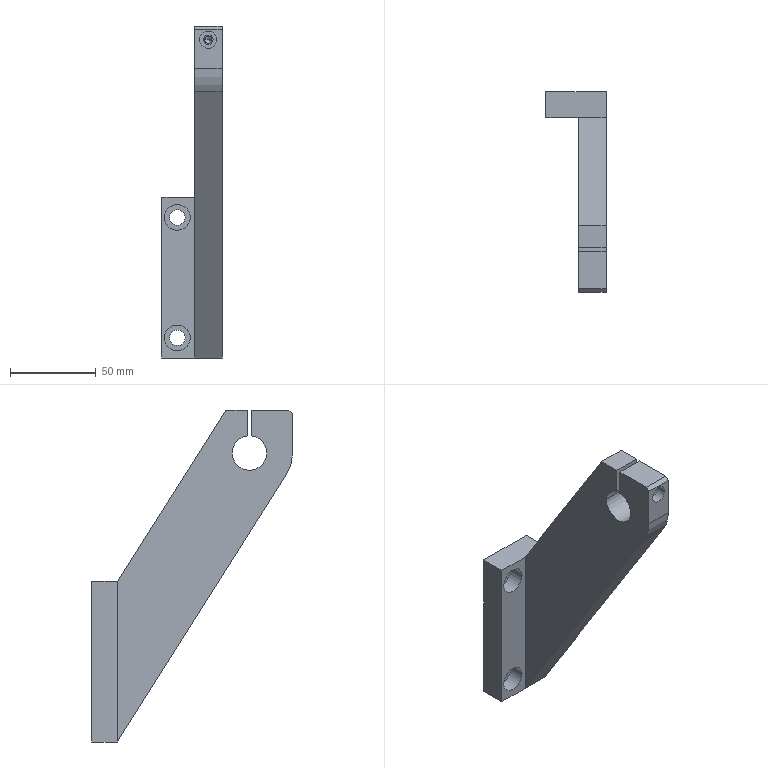Part | NX | features 0004 2 | 1 solid | 38 faces | box 35 x 116.8 x 193.095 mm | volume 171641 mm3 | plane 18 | cylinder 18 | cone 2 | commonest cylinder face diameters 9 x4 15 x4 20 x3 4.2 x2 5.5 x2 10 x2
STEP:
#1=CARTESIAN_POINT('',(-184.3,-184.,-863.625));
#2=VERTEX_POINT('',#1);
#3=CARTESIAN_POINT('',(-168.3,-184.,-863.625));
#4=VERTEX_POINT('',#3);
#5=CARTESIAN_POINT('',(-184.3,-184.,-863.625));
#6=DIRECTION('',(1.,0.,0.));
#7=VECTOR('',#6,1000.);
#8=LINE('',#5,#7);
#9=EDGE_CURVE('',#2,#4,#8,.T.);
#10=ORIENTED_EDGE('',*,*,#9,.T.);
#11=CARTESIAN_POINT('',(-168.3,-281.925,-708.899));
#12=VERTEX_POINT('',#11);
#13=CARTESIAN_POINT('',(-168.3,-281.925,-708.899));
#14=DIRECTION('',(0.,0.5348,-0.845));
#15=VECTOR('',#14,1000.);
#16=LINE('',#13,#15);
#17=EDGE_CURVE('',#12,#4,#16,.T.);
#18=ORIENTED_EDGE('',*,*,#17,.F.);
#19=CARTESIAN_POINT('',(-184.3,-281.925,-708.899));
#20=VERTEX_POINT('',#19);
#21=CARTESIAN_POINT('',(-184.3,-281.925,-708.899));
#22=DIRECTION('',(1.,0.,0.));
#23=VECTOR('',#22,1000.);
#24=LINE('',#21,#23);
#25=EDGE_CURVE('',#20,#12,#24,.T.);
#26=ORIENTED_EDGE('',*,*,#25,.F.);
#27=CARTESIAN_POINT('',(-184.3,-184.,-863.625));
#28=DIRECTION('',(0.,-0.5348,0.845));
#29=VECTOR('',#28,1000.);
#30=LINE('',#27,#29);
#31=EDGE_CURVE('',#2,#20,#30,.T.);
#32=ORIENTED_EDGE('',*,*,#31,.F.);
#33=EDGE_LOOP('',(#10,#18,#26,#32));
#34=FACE_BOUND('',#33,.T.);
#35=CARTESIAN_POINT('',(-168.3,-281.925,-708.899));
#36=DIRECTION('',(0.,0.845,0.5348));
#37=DIRECTION('',(0.,0.5348,-0.845));
#38=AXIS2_PLACEMENT_3D('',#35,#36,#37);
#39=PLANE('',#38);
#40=ADVANCED_FACE('',(#34),#39,.F.);
#41=ORIENTED_EDGE('',*,*,#25,.T.);
#42=CARTESIAN_POINT('',(-168.3,-285.8,-695.529));
#43=VERTEX_POINT('',#42);
#44=CARTESIAN_POINT('',(-168.3,-260.8,-695.529));
#45=DIRECTION('',(1.,0.,0.));
#46=DIRECTION('',(0.,-1.,0.));
#47=AXIS2_PLACEMENT_3D('',#44,#45,#46);
#48=CIRCLE('',#47,25.);
#49=EDGE_CURVE('',#43,#12,#48,.T.);
#50=ORIENTED_EDGE('',*,*,#49,.F.);
#51=CARTESIAN_POINT('',(-184.3,-285.8,-695.529));
#52=VERTEX_POINT('',#51);
#53=CARTESIAN_POINT('',(-168.3,-285.8,-695.529));
#54=DIRECTION('',(-1.,0.,0.));
#55=VECTOR('',#54,1000.);
#56=LINE('',#53,#55);
#57=EDGE_CURVE('',#43,#52,#56,.T.);
#58=ORIENTED_EDGE('',*,*,#57,.T.);
#59=CARTESIAN_POINT('',(-184.3,-260.8,-695.529));
#60=DIRECTION('',(-1.,0.,0.));
#61=DIRECTION('',(0.,-0.845,-0.5348));
#62=AXIS2_PLACEMENT_3D('',#59,#60,#61);
#63=CIRCLE('',#62,25.);
#64=EDGE_CURVE('',#20,#52,#63,.T.);
#65=ORIENTED_EDGE('',*,*,#64,.F.);
#66=EDGE_LOOP('',(#41,#50,#58,#65));
#67=FACE_BOUND('',#66,.T.);
#68=CARTESIAN_POINT('',(-168.3,-260.8,-695.529));
#69=DIRECTION('',(-1.,0.,0.));
#70=DIRECTION('',(0.,1.,0.));
#71=AXIS2_PLACEMENT_3D('',#68,#69,#70);
#72=CYLINDRICAL_SURFACE('',#71,25.);
#73=ADVANCED_FACE('',(#67),#72,.T.);
#74=CARTESIAN_POINT('',(-181.3,-280.1,-678.529));
#75=VERTEX_POINT('',#74);
#76=CARTESIAN_POINT('',(-171.3,-280.1,-678.529));
#77=VERTEX_POINT('',#76);
#78=CARTESIAN_POINT('',(-176.3,-280.1,-678.529));
#79=DIRECTION('',(0.,-1.,0.));
#80=DIRECTION('',(-1.,0.,0.));
#81=AXIS2_PLACEMENT_3D('',#78,#79,#80);
#82=CIRCLE('',#81,5.);
#83=EDGE_CURVE('',#75,#77,#82,.T.);
#84=ORIENTED_EDGE('',*,*,#83,.F.);
#85=CARTESIAN_POINT('',(-181.3,-285.8,-678.529));
#86=VERTEX_POINT('',#85);
#87=CARTESIAN_POINT('',(-181.3,-285.8,-678.529));
#88=DIRECTION('',(0.,1.,0.));
#89=VECTOR('',#88,1000.);
#90=LINE('',#87,#89);
#91=EDGE_CURVE('',#86,#75,#90,.T.);
#92=ORIENTED_EDGE('',*,*,#91,.F.);
#93=CARTESIAN_POINT('',(-171.3,-285.8,-678.529));
#94=VERTEX_POINT('',#93);
#95=CARTESIAN_POINT('',(-176.3,-285.8,-678.529));
#96=DIRECTION('',(0.,1.,0.));
#97=DIRECTION('',(1.,0.,0.));
#98=AXIS2_PLACEMENT_3D('',#95,#96,#97);
#99=CIRCLE('',#98,5.);
#100=EDGE_CURVE('',#94,#86,#99,.T.);
#101=ORIENTED_EDGE('',*,*,#100,.F.);
#102=CARTESIAN_POINT('',(-171.3,-285.8,-678.529));
#103=DIRECTION('',(0.,1.,0.));
#104=VECTOR('',#103,1000.);
#105=LINE('',#102,#104);
#106=EDGE_CURVE('',#77,#94,#105,.F.);
#107=ORIENTED_EDGE('',*,*,#106,.F.);
#108=EDGE_LOOP('',(#84,#92,#101,#107));
#109=FACE_BOUND('',#108,.T.);
#110=CARTESIAN_POINT('',(-176.3,-285.8,-678.529));
#111=DIRECTION('',(0.,-1.,0.));
#112=DIRECTION('',(-1.,0.,0.));
#113=AXIS2_PLACEMENT_3D('',#110,#111,#112);
#114=CYLINDRICAL_SURFACE('',#113,5.);
#115=ADVANCED_FACE('',(#109),#114,.F.);
#116=ORIENTED_EDGE('',*,*,#106,.T.);
#117=CARTESIAN_POINT('',(-176.3,-285.8,-678.529));
#118=DIRECTION('',(0.,1.,0.));
#119=DIRECTION('',(-1.,0.,0.));
#120=AXIS2_PLACEMENT_3D('',#117,#118,#119);
#121=CIRCLE('',#120,5.);
#122=EDGE_CURVE('',#86,#94,#121,.T.);
#123=ORIENTED_EDGE('',*,*,#122,.F.);
#124=ORIENTED_EDGE('',*,*,#91,.T.);
#125=CARTESIAN_POINT('',(-176.3,-280.1,-678.529));
#126=DIRECTION('',(0.,-1.,0.));
#127=DIRECTION('',(1.,0.,0.));
#128=AXIS2_PLACEMENT_3D('',#125,#126,#127);
#129=CIRCLE('',#128,5.);
#130=EDGE_CURVE('',#77,#75,#129,.T.);
#131=ORIENTED_EDGE('',*,*,#130,.F.);
#132=EDGE_LOOP('',(#116,#123,#124,#131));
#133=FACE_BOUND('',#132,.T.);
#134=CARTESIAN_POINT('',(-176.3,-285.8,-678.529));
#135=DIRECTION('',(0.,-1.,0.));
#136=DIRECTION('',(-1.,0.,0.));
#137=AXIS2_PLACEMENT_3D('',#134,#135,#136);
#138=CYLINDRICAL_SURFACE('',#137,5.);
#139=ADVANCED_FACE('',(#133),#138,.F.);
#140=CARTESIAN_POINT('',(-173.55,-280.1,-678.529));
#141=VERTEX_POINT('',#140);
#142=CARTESIAN_POINT('',(-179.05,-280.1,-678.529));
#143=VERTEX_POINT('',#142);
#144=CARTESIAN_POINT('',(-176.3,-280.1,-678.529));
#145=DIRECTION('',(0.,1.,0.));
#146=DIRECTION('',(1.,0.,0.));
#147=AXIS2_PLACEMENT_3D('',#144,#145,#146);
#148=CIRCLE('',#147,2.75);
#149=EDGE_CURVE('',#141,#143,#148,.T.);
#150=ORIENTED_EDGE('',*,*,#149,.T.);
#151=CARTESIAN_POINT('',(-176.3,-280.1,-678.529));
#152=DIRECTION('',(0.,1.,0.));
#153=DIRECTION('',(-1.,0.,0.));
#154=AXIS2_PLACEMENT_3D('',#151,#152,#153);
#155=CIRCLE('',#154,2.75);
#156=EDGE_CURVE('',#143,#141,#155,.T.);
#157=ORIENTED_EDGE('',*,*,#156,.T.);
#158=EDGE_LOOP('',(#150,#157));
#159=FACE_BOUND('',#158,.T.);
#160=ORIENTED_EDGE('',*,*,#83,.T.);
#161=ORIENTED_EDGE('',*,*,#130,.T.);
#162=EDGE_LOOP('',(#160,#161));
#163=FACE_BOUND('',#162,.T.);
#164=CARTESIAN_POINT('',(-176.3,-280.1,-675.779));
#165=DIRECTION('',(0.,1.,0.));
#166=DIRECTION('',(1.,0.,0.));
#167=AXIS2_PLACEMENT_3D('',#164,#165,#166);
#168=PLANE('',#167);
#169=ADVANCED_FACE('',(#159,#163),#168,.F.);
#170=CARTESIAN_POINT('',(-173.55,-262.05,-678.529));
#171=VERTEX_POINT('',#170);
#172=CARTESIAN_POINT('',(-173.55,-280.1,-678.529));
#173=DIRECTION('',(0.,1.,0.));
#174=VECTOR('',#173,1000.);
#175=LINE('',#172,#174);
#176=EDGE_CURVE('',#171,#141,#175,.F.);
#177=ORIENTED_EDGE('',*,*,#176,.T.);
#178=ORIENTED_EDGE('',*,*,#156,.F.);
#179=CARTESIAN_POINT('',(-179.05,-262.05,-678.529));
#180=VERTEX_POINT('',#179);
#181=CARTESIAN_POINT('',(-179.05,-280.1,-678.529));
#182=DIRECTION('',(0.,1.,0.));
#183=VECTOR('',#182,1000.);
#184=LINE('',#181,#183);
#185=EDGE_CURVE('',#143,#180,#184,.T.);
#186=ORIENTED_EDGE('',*,*,#185,.T.);
#187=CARTESIAN_POINT('',(-176.3,-262.05,-678.529));
#188=DIRECTION('',(0.,-1.,0.));
#189=DIRECTION('',(1.,0.,0.));
#190=AXIS2_PLACEMENT_3D('',#187,#188,#189);
#191=CIRCLE('',#190,2.75);
#192=EDGE_CURVE('',#171,#180,#191,.T.);
#193=ORIENTED_EDGE('',*,*,#192,.F.);
#194=EDGE_LOOP('',(#177,#178,#186,#193));
#195=FACE_BOUND('',#194,.T.);
#196=CARTESIAN_POINT('',(-176.3,-285.8,-678.529));
#197=DIRECTION('',(0.,-1.,0.));
#198=DIRECTION('',(-1.,0.,0.));
#199=AXIS2_PLACEMENT_3D('',#196,#197,#198);
#200=CYLINDRICAL_SURFACE('',#199,2.75);
#201=ADVANCED_FACE('',(#195),#200,.F.);
#202=CARTESIAN_POINT('',(-176.3,-262.05,-678.529));
#203=DIRECTION('',(0.,-1.,0.));
#204=DIRECTION('',(-1.,0.,0.));
#205=AXIS2_PLACEMENT_3D('',#202,#203,#204);
#206=CIRCLE('',#205,2.75);
#207=EDGE_CURVE('',#180,#171,#206,.T.);
#208=ORIENTED_EDGE('',*,*,#207,.F.);
#209=ORIENTED_EDGE('',*,*,#185,.F.);
#210=ORIENTED_EDGE('',*,*,#149,.F.);
#211=ORIENTED_EDGE('',*,*,#176,.F.);
#212=EDGE_LOOP('',(#208,#209,#210,#211));
#213=FACE_BOUND('',#212,.T.);
#214=CARTESIAN_POINT('',(-176.3,-285.8,-678.529));
#215=DIRECTION('',(0.,-1.,0.));
#216=DIRECTION('',(-1.,0.,0.));
#217=AXIS2_PLACEMENT_3D('',#214,#215,#216);
#218=CYLINDRICAL_SURFACE('',#217,2.75);
#219=ADVANCED_FACE('',(#213),#218,.F.);
#220=CARTESIAN_POINT('',(-178.4,-247.15,-678.529));
#221=VERTEX_POINT('',#220);
#222=CARTESIAN_POINT('',(-174.2,-247.15,-678.529));
#223=VERTEX_POINT('',#222);
#224=CARTESIAN_POINT('',(-176.3,-247.15,-678.529));
#225=DIRECTION('',(0.,-1.,0.));
#226=DIRECTION('',(-1.,0.,0.));
#227=AXIS2_PLACEMENT_3D('',#224,#225,#226);
#228=CIRCLE('',#227,2.1);
#229=EDGE_CURVE('',#221,#223,#228,.T.);
#230=ORIENTED_EDGE('',*,*,#229,.F.);
#231=CARTESIAN_POINT('',(-178.4,-259.55,-678.529));
#232=VERTEX_POINT('',#231);
#233=CARTESIAN_POINT('',(-178.4,-259.55,-678.529));
#234=DIRECTION('',(0.,1.,0.));
#235=VECTOR('',#234,1000.);
#236=LINE('',#233,#235);
#237=EDGE_CURVE('',#232,#221,#236,.T.);
#238=ORIENTED_EDGE('',*,*,#237,.F.);
#239=CARTESIAN_POINT('',(-174.2,-259.55,-678.529));
#240=VERTEX_POINT('',#239);
#241=CARTESIAN_POINT('',(-176.3,-259.55,-678.529));
#242=DIRECTION('',(0.,1.,0.));
#243=DIRECTION('',(1.,0.,0.));
#244=AXIS2_PLACEMENT_3D('',#241,#242,#243);
#245=CIRCLE('',#244,2.1);
#246=EDGE_CURVE('',#240,#232,#245,.T.);
#247=ORIENTED_EDGE('',*,*,#246,.F.);
#248=CARTESIAN_POINT('',(-174.2,-259.55,-678.529));
#249=DIRECTION('',(0.,1.,0.));
#250=VECTOR('',#249,1000.);
#251=LINE('',#248,#250);
#252=EDGE_CURVE('',#223,#240,#251,.F.);
#253=ORIENTED_EDGE('',*,*,#252,.F.);
#254=EDGE_LOOP('',(#230,#238,#247,#253));
#255=FACE_BOUND('',#254,.T.);
#256=CARTESIAN_POINT('',(-176.3,-259.55,-678.529));
#257=DIRECTION('',(0.,-1.,0.));
#258=DIRECTION('',(-1.,0.,0.));
#259=AXIS2_PLACEMENT_3D('',#256,#257,#258);
#260=CYLINDRICAL_SURFACE('',#259,2.1);
#261=ADVANCED_FACE('',(#255),#260,.F.);
#262=CARTESIAN_POINT('',(-176.3,-245.888,-678.529));
#263=VERTEX_POINT('',#262);
#264=CARTESIAN_POINT('',(-178.4,-247.15,-678.529));
#265=DIRECTION('',(0.8572,0.515,0.));
#266=VECTOR('',#265,1000.);
#267=LINE('',#264,#266);
#268=EDGE_CURVE('',#263,#221,#267,.F.);
#269=ORIENTED_EDGE('',*,*,#268,.T.);
#270=ORIENTED_EDGE('',*,*,#229,.T.);
#271=CARTESIAN_POINT('',(-174.2,-247.15,-678.529));
#272=DIRECTION('',(-0.8572,0.515,0.));
#273=VECTOR('',#272,1000.);
#274=LINE('',#271,#273);
#275=EDGE_CURVE('',#223,#263,#274,.T.);
#276=ORIENTED_EDGE('',*,*,#275,.T.);
#277=EDGE_LOOP('',(#269,#270,#276));
#278=FACE_BOUND('',#277,.T.);
#279=CARTESIAN_POINT('',(-176.3,-245.888,-678.529));
#280=DIRECTION('',(0.,-1.,0.));
#281=DIRECTION('',(-1.,0.,0.));
#282=AXIS2_PLACEMENT_3D('',#279,#280,#281);
#283=CONICAL_SURFACE('',#282,0.,1.03);
#284=ADVANCED_FACE('',(#278),#283,.F.);
#285=ORIENTED_EDGE('',*,*,#275,.F.);
#286=CARTESIAN_POINT('',(-176.3,-247.15,-678.529));
#287=DIRECTION('',(0.,-1.,0.));
#288=DIRECTION('',(1.,0.,0.));
#289=AXIS2_PLACEMENT_3D('',#286,#287,#288);
#290=CIRCLE('',#289,2.1);
#291=EDGE_CURVE('',#223,#221,#290,.T.);
#292=ORIENTED_EDGE('',*,*,#291,.T.);
#293=ORIENTED_EDGE('',*,*,#268,.F.);
#294=EDGE_LOOP('',(#285,#292,#293));
#295=FACE_BOUND('',#294,.T.);
#296=CARTESIAN_POINT('',(-176.3,-245.888,-678.529));
#297=DIRECTION('',(0.,-1.,0.));
#298=DIRECTION('',(-1.,0.,0.));
#299=AXIS2_PLACEMENT_3D('',#296,#297,#298);
#300=CONICAL_SURFACE('',#299,0.,1.03);
#301=ADVANCED_FACE('',(#295),#300,.F.);
#302=ORIENTED_EDGE('',*,*,#252,.T.);
#303=CARTESIAN_POINT('',(-176.3,-259.55,-678.529));
#304=DIRECTION('',(0.,1.,0.));
#305=DIRECTION('',(-1.,0.,0.));
#306=AXIS2_PLACEMENT_3D('',#303,#304,#305);
#307=CIRCLE('',#306,2.1);
#308=EDGE_CURVE('',#232,#240,#307,.T.);
#309=ORIENTED_EDGE('',*,*,#308,.F.);
#310=ORIENTED_EDGE('',*,*,#237,.T.);
#311=ORIENTED_EDGE('',*,*,#291,.F.);
#312=EDGE_LOOP('',(#302,#309,#310,#311));
#313=FACE_BOUND('',#312,.T.);
#314=CARTESIAN_POINT('',(-176.3,-259.55,-678.529));
#315=DIRECTION('',(0.,-1.,0.));
#316=DIRECTION('',(-1.,0.,0.));
#317=AXIS2_PLACEMENT_3D('',#314,#315,#316);
#318=CYLINDRICAL_SURFACE('',#317,2.1);
#319=ADVANCED_FACE('',(#313),#318,.F.);
#320=CARTESIAN_POINT('',(-201.8,-175.,-781.877));
#321=VERTEX_POINT('',#320);
#322=CARTESIAN_POINT('',(-186.8,-175.,-781.877));
#323=VERTEX_POINT('',#322);
#324=CARTESIAN_POINT('',(-194.3,-175.,-781.877));
#325=DIRECTION('',(0.,-1.,0.));
#326=DIRECTION('',(-1.,0.,0.));
#327=AXIS2_PLACEMENT_3D('',#324,#325,#326);
#328=CIRCLE('',#327,7.5);
#329=EDGE_CURVE('',#321,#323,#328,.T.);
#330=ORIENTED_EDGE('',*,*,#329,.F.);
#331=CARTESIAN_POINT('',(-201.8,-184.,-781.877));
#332=VERTEX_POINT('',#331);
#333=CARTESIAN_POINT('',(-201.8,-184.,-781.877));
#334=DIRECTION('',(0.,1.,0.));
#335=VECTOR('',#334,1000.);
#336=LINE('',#333,#335);
#337=EDGE_CURVE('',#332,#321,#336,.T.);
#338=ORIENTED_EDGE('',*,*,#337,.F.);
#339=CARTESIAN_POINT('',(-186.8,-184.,-781.877));
#340=VERTEX_POINT('',#339);
#341=CARTESIAN_POINT('',(-194.3,-184.,-781.877));
#342=DIRECTION('',(0.,1.,0.));
#343=DIRECTION('',(1.,0.,0.));
#344=AXIS2_PLACEMENT_3D('',#341,#342,#343);
#345=CIRCLE('',#344,7.5);
#346=EDGE_CURVE('',#340,#332,#345,.T.);
#347=ORIENTED_EDGE('',*,*,#346,.F.);
#348=CARTESIAN_POINT('',(-186.8,-184.,-781.877));
#349=DIRECTION('',(0.,1.,0.));
#350=VECTOR('',#349,1000.);
#351=LINE('',#348,#350);
#352=EDGE_CURVE('',#323,#340,#351,.F.);
#353=ORIENTED_EDGE('',*,*,#352,.F.);
#354=EDGE_LOOP('',(#330,#338,#347,#353));
#355=FACE_BOUND('',#354,.T.);
#356=CARTESIAN_POINT('',(-194.3,-184.,-781.877));
#357=DIRECTION('',(0.,-1.,0.));
#358=DIRECTION('',(-1.,0.,0.));
#359=AXIS2_PLACEMENT_3D('',#356,#357,#358);
#360=CYLINDRICAL_SURFACE('',#359,7.5);
#361=ADVANCED_FACE('',(#355),#360,.F.);
#362=ORIENTED_EDGE('',*,*,#352,.T.);
#363=CARTESIAN_POINT('',(-194.3,-184.,-781.877));
#364=DIRECTION('',(0.,1.,0.));
#365=DIRECTION('',(-1.,0.,0.));
#366=AXIS2_PLACEMENT_3D('',#363,#364,#365);
#367=CIRCLE('',#366,7.5);
#368=EDGE_CURVE('',#332,#340,#367,.T.);
#369=ORIENTED_EDGE('',*,*,#368,.F.);
#370=ORIENTED_EDGE('',*,*,#337,.T.);
#371=CARTESIAN_POINT('',(-194.3,-175.,-781.877));
#372=DIRECTION('',(0.,-1.,0.));
#373=DIRECTION('',(1.,0.,0.));
#374=AXIS2_PLACEMENT_3D('',#371,#372,#373);
#375=CIRCLE('',#374,7.5);
#376=EDGE_CURVE('',#323,#321,#375,.T.);
#377=ORIENTED_EDGE('',*,*,#376,.F.);
#378=EDGE_LOOP('',(#362,#369,#370,#377));
#379=FACE_BOUND('',#378,.T.);
#380=CARTESIAN_POINT('',(-194.3,-184.,-781.877));
#381=DIRECTION('',(0.,-1.,0.));
#382=DIRECTION('',(-1.,0.,0.));
#383=AXIS2_PLACEMENT_3D('',#380,#381,#382);
#384=CYLINDRICAL_SURFACE('',#383,7.5);
#385=ADVANCED_FACE('',(#379),#384,.F.);
#386=CARTESIAN_POINT('',(-189.8,-175.,-781.877));
#387=VERTEX_POINT('',#386);
#388=CARTESIAN_POINT('',(-198.8,-175.,-781.877));
#389=VERTEX_POINT('',#388);
#390=CARTESIAN_POINT('',(-194.3,-175.,-781.877));
#391=DIRECTION('',(0.,1.,0.));
#392=DIRECTION('',(1.,0.,0.));
#393=AXIS2_PLACEMENT_3D('',#390,#391,#392);
#394=CIRCLE('',#393,4.5);
#395=EDGE_CURVE('',#387,#389,#394,.T.);
#396=ORIENTED_EDGE('',*,*,#395,.T.);
#397=CARTESIAN_POINT('',(-194.3,-175.,-781.877));
#398=DIRECTION('',(0.,1.,0.));
#399=DIRECTION('',(-1.,0.,0.));
#400=AXIS2_PLACEMENT_3D('',#397,#398,#399);
#401=CIRCLE('',#400,4.5);
#402=EDGE_CURVE('',#389,#387,#401,.T.);
#403=ORIENTED_EDGE('',*,*,#402,.T.);
#404=EDGE_LOOP('',(#396,#403));
#405=FACE_BOUND('',#404,.T.);
#406=ORIENTED_EDGE('',*,*,#329,.T.);
#407=ORIENTED_EDGE('',*,*,#376,.T.);
#408=EDGE_LOOP('',(#406,#407));
#409=FACE_BOUND('',#408,.T.);
#410=CARTESIAN_POINT('',(-194.3,-175.,-777.377));
#411=DIRECTION('',(0.,1.,0.));
#412=DIRECTION('',(1.,0.,0.));
#413=AXIS2_PLACEMENT_3D('',#410,#411,#412);
#414=PLANE('',#413);
#415=ADVANCED_FACE('',(#405,#409),#414,.F.);
#416=CARTESIAN_POINT('',(-198.8,-169.,-781.877));
#417=VERTEX_POINT('',#416);
#418=CARTESIAN_POINT('',(-189.8,-169.,-781.877));
#419=VERTEX_POINT('',#418);
#420=CARTESIAN_POINT('',(-194.3,-169.,-781.877));
#421=DIRECTION('',(0.,-1.,0.));
#422=DIRECTION('',(-1.,0.,0.));
#423=AXIS2_PLACEMENT_3D('',#420,#421,#422);
#424=CIRCLE('',#423,4.5);
#425=EDGE_CURVE('',#417,#419,#424,.T.);
#426=ORIENTED_EDGE('',*,*,#425,.F.);
#427=CARTESIAN_POINT('',(-198.8,-175.,-781.877));
#428=DIRECTION('',(0.,1.,0.));
#429=VECTOR('',#428,1000.);
#430=LINE('',#427,#429);
#431=EDGE_CURVE('',#417,#389,#430,.F.);
#432=ORIENTED_EDGE('',*,*,#431,.T.);
#433=ORIENTED_EDGE('',*,*,#395,.F.);
#434=CARTESIAN_POINT('',(-189.8,-175.,-781.877));
#435=DIRECTION('',(0.,1.,0.));
#436=VECTOR('',#435,1000.);
#437=LINE('',#434,#436);
#438=EDGE_CURVE('',#387,#419,#437,.T.);
#439=ORIENTED_EDGE('',*,*,#438,.T.);
#440=EDGE_LOOP('',(#426,#432,#433,#439));
#441=FACE_BOUND('',#440,.T.);
#442=CARTESIAN_POINT('',(-194.3,-184.,-781.877));
#443=DIRECTION('',(0.,-1.,0.));
#444=DIRECTION('',(-1.,0.,0.));
#445=AXIS2_PLACEMENT_3D('',#442,#443,#444);
#446=CYLINDRICAL_SURFACE('',#445,4.5);
#447=ADVANCED_FACE('',(#441),#446,.F.);
#448=ORIENTED_EDGE('',*,*,#438,.F.);
#449=ORIENTED_EDGE('',*,*,#402,.F.);
#450=ORIENTED_EDGE('',*,*,#431,.F.);
#451=CARTESIAN_POINT('',(-194.3,-169.,-781.877));
#452=DIRECTION('',(0.,-1.,0.));
#453=DIRECTION('',(1.,0.,0.));
#454=AXIS2_PLACEMENT_3D('',#451,#452,#453);
#455=CIRCLE('',#454,4.5);
#456=EDGE_CURVE('',#419,#417,#455,.T.);
#457=ORIENTED_EDGE('',*,*,#456,.F.);
#458=EDGE_LOOP('',(#448,#449,#450,#457));
#459=FACE_BOUND('',#458,.T.);
#460=CARTESIAN_POINT('',(-194.3,-184.,-781.877));
#461=DIRECTION('',(0.,-1.,0.));
#462=DIRECTION('',(-1.,0.,0.));
#463=AXIS2_PLACEMENT_3D('',#460,#461,#462);
#464=CYLINDRICAL_SURFACE('',#463,4.5);
#465=ADVANCED_FACE('',(#459),#464,.F.);
#466=CARTESIAN_POINT('',(-201.8,-175.,-851.877));
#467=VERTEX_POINT('',#466);
#468=CARTESIAN_POINT('',(-186.8,-175.,-851.877));
#469=VERTEX_POINT('',#468);
#470=CARTESIAN_POINT('',(-194.3,-175.,-851.877));
#471=DIRECTION('',(0.,-1.,0.));
#472=DIRECTION('',(-1.,0.,0.));
#473=AXIS2_PLACEMENT_3D('',#470,#471,#472);
#474=CIRCLE('',#473,7.5);
#475=EDGE_CURVE('',#467,#469,#474,.T.);
#476=ORIENTED_EDGE('',*,*,#475,.F.);
#477=CARTESIAN_POINT('',(-201.8,-184.,-851.877));
#478=VERTEX_POINT('',#477);
#479=CARTESIAN_POINT('',(-201.8,-184.,-851.877));
#480=DIRECTION('',(0.,1.,0.));
#481=VECTOR('',#480,1000.);
#482=LINE('',#479,#481);
#483=EDGE_CURVE('',#467,#478,#482,.F.);
#484=ORIENTED_EDGE('',*,*,#483,.T.);
#485=CARTESIAN_POINT('',(-186.8,-184.,-851.877));
#486=VERTEX_POINT('',#485);
#487=CARTESIAN_POINT('',(-194.3,-184.,-851.877));
#488=DIRECTION('',(0.,1.,0.));
#489=DIRECTION('',(1.,0.,0.));
#490=AXIS2_PLACEMENT_3D('',#487,#488,#489);
#491=CIRCLE('',#490,7.5);
#492=EDGE_CURVE('',#486,#478,#491,.T.);
#493=ORIENTED_EDGE('',*,*,#492,.F.);
#494=CARTESIAN_POINT('',(-186.8,-184.,-851.877));
#495=DIRECTION('',(0.,1.,0.));
#496=VECTOR('',#495,1000.);
#497=LINE('',#494,#496);
#498=EDGE_CURVE('',#486,#469,#497,.T.);
#499=ORIENTED_EDGE('',*,*,#498,.T.);
#500=EDGE_LOOP('',(#476,#484,#493,#499));
#501=FACE_BOUND('',#500,.T.);
#502=CARTESIAN_POINT('',(-194.3,-184.,-851.877));
#503=DIRECTION('',(0.,-1.,0.));
#504=DIRECTION('',(-1.,0.,0.));
#505=AXIS2_PLACEMENT_3D('',#502,#503,#504);
#506=CYLINDRICAL_SURFACE('',#505,7.5);
#507=ADVANCED_FACE('',(#501),#506,.F.);
#508=ORIENTED_EDGE('',*,*,#498,.F.);
#509=CARTESIAN_POINT('',(-194.3,-184.,-851.877));
#510=DIRECTION('',(0.,1.,0.));
#511=DIRECTION('',(-1.,0.,0.));
#512=AXIS2_PLACEMENT_3D('',#509,#510,#511);
#513=CIRCLE('',#512,7.5);
#514=EDGE_CURVE('',#478,#486,#513,.T.);
#515=ORIENTED_EDGE('',*,*,#514,.F.);
#516=ORIENTED_EDGE('',*,*,#483,.F.);
#517=CARTESIAN_POINT('',(-194.3,-175.,-851.877));
#518=DIRECTION('',(0.,-1.,0.));
#519=DIRECTION('',(1.,0.,0.));
#520=AXIS2_PLACEMENT_3D('',#517,#518,#519);
#521=CIRCLE('',#520,7.5);
#522=EDGE_CURVE('',#469,#467,#521,.T.);
#523=ORIENTED_EDGE('',*,*,#522,.F.);
#524=EDGE_LOOP('',(#508,#515,#516,#523));
#525=FACE_BOUND('',#524,.T.);
#526=CARTESIAN_POINT('',(-194.3,-184.,-851.877));
#527=DIRECTION('',(0.,-1.,0.));
#528=DIRECTION('',(-1.,0.,0.));
#529=AXIS2_PLACEMENT_3D('',#526,#527,#528);
#530=CYLINDRICAL_SURFACE('',#529,7.5);
#531=ADVANCED_FACE('',(#525),#530,.F.);
#532=CARTESIAN_POINT('',(-189.8,-175.,-851.877));
#533=VERTEX_POINT('',#532);
#534=CARTESIAN_POINT('',(-198.8,-175.,-851.877));
#535=VERTEX_POINT('',#534);
#536=CARTESIAN_POINT('',(-194.3,-175.,-851.877));
#537=DIRECTION('',(0.,1.,0.));
#538=DIRECTION('',(1.,0.,0.));
#539=AXIS2_PLACEMENT_3D('',#536,#537,#538);
#540=CIRCLE('',#539,4.5);
#541=EDGE_CURVE('',#533,#535,#540,.T.);
#542=ORIENTED_EDGE('',*,*,#541,.T.);
#543=CARTESIAN_POINT('',(-194.3,-175.,-851.877));
#544=DIRECTION('',(0.,1.,0.));
#545=DIRECTION('',(-1.,0.,0.));
#546=AXIS2_PLACEMENT_3D('',#543,#544,#545);
#547=CIRCLE('',#546,4.5);
#548=EDGE_CURVE('',#535,#533,#547,.T.);
#549=ORIENTED_EDGE('',*,*,#548,.T.);
#550=EDGE_LOOP('',(#542,#549));
#551=FACE_BOUND('',#550,.T.);
#552=ORIENTED_EDGE('',*,*,#475,.T.);
#553=ORIENTED_EDGE('',*,*,#522,.T.);
#554=EDGE_LOOP('',(#552,#553));
#555=FACE_BOUND('',#554,.T.);
#556=CARTESIAN_POINT('',(-194.3,-175.,-847.377));
#557=DIRECTION('',(0.,1.,0.));
#558=DIRECTION('',(1.,0.,0.));
#559=AXIS2_PLACEMENT_3D('',#556,#557,#558);
#560=PLANE('',#559);
#561=ADVANCED_FACE('',(#551,#555),#560,.F.);
#562=CARTESIAN_POINT('',(-198.8,-169.,-851.877));
#563=VERTEX_POINT('',#562);
#564=CARTESIAN_POINT('',(-189.8,-169.,-851.877));
#565=VERTEX_POINT('',#564);
#566=CARTESIAN_POINT('',(-194.3,-169.,-851.877));
#567=DIRECTION('',(0.,-1.,0.));
#568=DIRECTION('',(-1.,0.,0.));
#569=AXIS2_PLACEMENT_3D('',#566,#567,#568);
#570=CIRCLE('',#569,4.5);
#571=EDGE_CURVE('',#563,#565,#570,.T.);
#572=ORIENTED_EDGE('',*,*,#571,.F.);
#573=CARTESIAN_POINT('',(-198.8,-175.,-851.877));
#574=DIRECTION('',(0.,1.,0.));
#575=VECTOR('',#574,1000.);
#576=LINE('',#573,#575);
#577=EDGE_CURVE('',#535,#563,#576,.T.);
#578=ORIENTED_EDGE('',*,*,#577,.F.);
#579=ORIENTED_EDGE('',*,*,#541,.F.);
#580=CARTESIAN_POINT('',(-189.8,-175.,-851.877));
#581=DIRECTION('',(0.,1.,0.));
#582=VECTOR('',#581,1000.);
#583=LINE('',#580,#582);
#584=EDGE_CURVE('',#565,#533,#583,.F.);
#585=ORIENTED_EDGE('',*,*,#584,.F.);
#586=EDGE_LOOP('',(#572,#578,#579,#585));
#587=FACE_BOUND('',#586,.T.);
#588=CARTESIAN_POINT('',(-194.3,-184.,-851.877));
#589=DIRECTION('',(0.,-1.,0.));
#590=DIRECTION('',(-1.,0.,0.));
#591=AXIS2_PLACEMENT_3D('',#588,#589,#590);
#592=CYLINDRICAL_SURFACE('',#591,4.5);
#593=ADVANCED_FACE('',(#587),#592,.F.);
#594=ORIENTED_EDGE('',*,*,#584,.T.);
#595=ORIENTED_EDGE('',*,*,#548,.F.);
#596=ORIENTED_EDGE('',*,*,#577,.T.);
#597=CARTESIAN_POINT('',(-194.3,-169.,-851.877));
#598=DIRECTION('',(0.,-1.,0.));
#599=DIRECTION('',(1.,0.,0.));
#600=AXIS2_PLACEMENT_3D('',#597,#598,#599);
#601=CIRCLE('',#600,4.5);
#602=EDGE_CURVE('',#565,#563,#601,.T.);
#603=ORIENTED_EDGE('',*,*,#602,.F.);
#604=EDGE_LOOP('',(#594,#595,#596,#603));
#605=FACE_BOUND('',#604,.T.);
#606=CARTESIAN_POINT('',(-194.3,-184.,-851.877));
#607=DIRECTION('',(0.,-1.,0.));
#608=DIRECTION('',(-1.,0.,0.));
#609=AXIS2_PLACEMENT_3D('',#606,#607,#608);
#610=CYLINDRICAL_SURFACE('',#609,4.5);
#611=ADVANCED_FACE('',(#605),#610,.F.);
#612=ORIENTED_EDGE('',*,*,#425,.T.);
#613=ORIENTED_EDGE('',*,*,#456,.T.);
#614=EDGE_LOOP('',(#612,#613));
#615=FACE_BOUND('',#614,.T.);
#616=ORIENTED_EDGE('',*,*,#571,.T.);
#617=ORIENTED_EDGE('',*,*,#602,.T.);
#618=EDGE_LOOP('',(#616,#617));
#619=FACE_BOUND('',#618,.T.);
#620=CARTESIAN_POINT('',(-168.3,-169.,-863.625));
#621=VERTEX_POINT('',#620);
#622=CARTESIAN_POINT('',(-203.3,-169.,-863.625));
#623=VERTEX_POINT('',#622);
#624=CARTESIAN_POINT('',(-168.3,-169.,-863.625));
#625=DIRECTION('',(-1.,0.,0.));
#626=VECTOR('',#625,1000.);
#627=LINE('',#624,#626);
#628=EDGE_CURVE('',#621,#623,#627,.T.);
#629=ORIENTED_EDGE('',*,*,#628,.T.);
#630=CARTESIAN_POINT('',(-203.3,-169.,-770.129));
#631=VERTEX_POINT('',#630);
#632=CARTESIAN_POINT('',(-203.3,-169.,-863.625));
#633=DIRECTION('',(0.,0.,1.));
#634=VECTOR('',#633,1000.);
#635=LINE('',#632,#634);
#636=EDGE_CURVE('',#623,#631,#635,.T.);
#637=ORIENTED_EDGE('',*,*,#636,.T.);
#638=CARTESIAN_POINT('',(-168.3,-169.,-770.129));
#639=VERTEX_POINT('',#638);
#640=CARTESIAN_POINT('',(-168.3,-169.,-770.129));
#641=DIRECTION('',(-1.,0.,0.));
#642=VECTOR('',#641,1000.);
#643=LINE('',#640,#642);
#644=EDGE_CURVE('',#639,#631,#643,.T.);
#645=ORIENTED_EDGE('',*,*,#644,.F.);
#646=CARTESIAN_POINT('',(-168.3,-169.,-863.625));
#647=DIRECTION('',(0.,0.,1.));
#648=VECTOR('',#647,1000.);
#649=LINE('',#646,#648);
#650=EDGE_CURVE('',#621,#639,#649,.T.);
#651=ORIENTED_EDGE('',*,*,#650,.F.);
#652=EDGE_LOOP('',(#629,#637,#645,#651));
#653=FACE_BOUND('',#652,.T.);
#654=CARTESIAN_POINT('',(-203.3,-169.,-770.129));
#655=DIRECTION('',(0.,1.,0.));
#656=DIRECTION('',(1.,0.,0.));
#657=AXIS2_PLACEMENT_3D('',#654,#655,#656);
#658=PLANE('',#657);
#659=ADVANCED_FACE('',(#615,#619,#653),#658,.T.);
#660=CARTESIAN_POINT('',(-203.3,-184.,-863.625));
#661=VERTEX_POINT('',#660);
#662=CARTESIAN_POINT('',(-203.3,-184.,-863.625));
#663=DIRECTION('',(0.,1.,0.));
#664=VECTOR('',#663,1000.);
#665=LINE('',#662,#664);
#666=EDGE_CURVE('',#661,#623,#665,.T.);
#667=ORIENTED_EDGE('',*,*,#666,.F.);
#668=CARTESIAN_POINT('',(-203.3,-184.,-770.129));
#669=VERTEX_POINT('',#668);
#670=CARTESIAN_POINT('',(-203.3,-184.,-770.129));
#671=DIRECTION('',(0.,0.,-1.));
#672=VECTOR('',#671,1000.);
#673=LINE('',#670,#672);
#674=EDGE_CURVE('',#669,#661,#673,.T.);
#675=ORIENTED_EDGE('',*,*,#674,.F.);
#676=CARTESIAN_POINT('',(-203.3,-169.,-770.129));
#677=DIRECTION('',(0.,-1.,0.));
#678=VECTOR('',#677,1000.);
#679=LINE('',#676,#678);
#680=EDGE_CURVE('',#631,#669,#679,.T.);
#681=ORIENTED_EDGE('',*,*,#680,.F.);
#682=ORIENTED_EDGE('',*,*,#636,.F.);
#683=EDGE_LOOP('',(#667,#675,#681,#682));
#684=FACE_BOUND('',#683,.T.);
#685=CARTESIAN_POINT('',(-203.3,-169.,-770.129));
#686=DIRECTION('',(1.,0.,0.));
#687=DIRECTION('',(0.,-1.,0.));
#688=AXIS2_PLACEMENT_3D('',#685,#686,#687);
#689=PLANE('',#688);
#690=ADVANCED_FACE('',(#684),#689,.F.);
#691=ORIENTED_EDGE('',*,*,#492,.T.);
#692=ORIENTED_EDGE('',*,*,#514,.T.);
#693=EDGE_LOOP('',(#691,#692));
#694=FACE_BOUND('',#693,.T.);
#695=ORIENTED_EDGE('',*,*,#346,.T.);
#696=ORIENTED_EDGE('',*,*,#368,.T.);
#697=EDGE_LOOP('',(#695,#696));
#698=FACE_BOUND('',#697,.T.);
#699=ORIENTED_EDGE('',*,*,#674,.T.);
#700=CARTESIAN_POINT('',(-184.3,-184.,-863.625));
#701=DIRECTION('',(-1.,0.,0.));
#702=VECTOR('',#701,1000.);
#703=LINE('',#700,#702);
#704=EDGE_CURVE('',#2,#661,#703,.T.);
#705=ORIENTED_EDGE('',*,*,#704,.F.);
#706=CARTESIAN_POINT('',(-184.3,-184.,-770.129));
#707=VERTEX_POINT('',#706);
#708=CARTESIAN_POINT('',(-184.3,-184.,-863.625));
#709=DIRECTION('',(0.,0.,1.));
#710=VECTOR('',#709,1000.);
#711=LINE('',#708,#710);
#712=EDGE_CURVE('',#2,#707,#711,.T.);
#713=ORIENTED_EDGE('',*,*,#712,.T.);
#714=CARTESIAN_POINT('',(-184.3,-184.,-770.129));
#715=DIRECTION('',(-1.,0.,0.));
#716=VECTOR('',#715,1000.);
#717=LINE('',#714,#716);
#718=EDGE_CURVE('',#707,#669,#717,.T.);
#719=ORIENTED_EDGE('',*,*,#718,.T.);
#720=EDGE_LOOP('',(#699,#705,#713,#719));
#721=FACE_BOUND('',#720,.T.);
#722=CARTESIAN_POINT('',(-203.3,-184.,-770.129));
#723=DIRECTION('',(0.,-1.,0.));
#724=DIRECTION('',(-1.,0.,0.));
#725=AXIS2_PLACEMENT_3D('',#722,#723,#724);
#726=PLANE('',#725);
#727=ADVANCED_FACE('',(#694,#698,#721),#726,.T.);
#728=ORIENTED_EDGE('',*,*,#644,.T.);
#729=ORIENTED_EDGE('',*,*,#680,.T.);
#730=ORIENTED_EDGE('',*,*,#718,.F.);
#731=CARTESIAN_POINT('',(-168.3,-184.,-770.129));
#732=VERTEX_POINT('',#731);
#733=CARTESIAN_POINT('',(-184.3,-184.,-770.129));
#734=DIRECTION('',(1.,0.,0.));
#735=VECTOR('',#734,1000.);
#736=LINE('',#733,#735);
#737=EDGE_CURVE('',#707,#732,#736,.T.);
#738=ORIENTED_EDGE('',*,*,#737,.T.);
#739=CARTESIAN_POINT('',(-168.3,-169.,-770.129));
#740=DIRECTION('',(0.,-1.,0.));
#741=VECTOR('',#740,1000.);
#742=LINE('',#739,#741);
#743=EDGE_CURVE('',#639,#732,#742,.T.);
#744=ORIENTED_EDGE('',*,*,#743,.F.);
#745=EDGE_LOOP('',(#728,#729,#730,#738,#744));
#746=FACE_BOUND('',#745,.T.);
#747=CARTESIAN_POINT('',(-203.3,-169.,-770.129));
#748=DIRECTION('',(0.,0.,1.));
#749=DIRECTION('',(1.,0.,0.));
#750=AXIS2_PLACEMENT_3D('',#747,#748,#749);
#751=PLANE('',#750);
#752=ADVANCED_FACE('',(#746),#751,.T.);
#753=CARTESIAN_POINT('',(-184.3,-247.036,-670.529));
#754=VERTEX_POINT('',#753);
#755=CARTESIAN_POINT('',(-168.3,-247.036,-670.529));
#756=VERTEX_POINT('',#755);
#757=CARTESIAN_POINT('',(-184.3,-247.036,-670.529));
#758=DIRECTION('',(1.,0.,0.));
#759=VECTOR('',#758,1000.);
#760=LINE('',#757,#759);
#761=EDGE_CURVE('',#754,#756,#760,.T.);
#762=ORIENTED_EDGE('',*,*,#761,.T.);
#763=CARTESIAN_POINT('',(-168.3,-184.,-770.129));
#764=DIRECTION('',(0.,-0.5348,0.845));
#765=VECTOR('',#764,1000.);
#766=LINE('',#763,#765);
#767=EDGE_CURVE('',#732,#756,#766,.T.);
#768=ORIENTED_EDGE('',*,*,#767,.F.);
#769=ORIENTED_EDGE('',*,*,#737,.F.);
#770=CARTESIAN_POINT('',(-184.3,-247.036,-670.529));
#771=DIRECTION('',(0.,0.5348,-0.845));
#772=VECTOR('',#771,1000.);
#773=LINE('',#770,#772);
#774=EDGE_CURVE('',#754,#707,#773,.T.);
#775=ORIENTED_EDGE('',*,*,#774,.F.);
#776=EDGE_LOOP('',(#762,#768,#769,#775));
#777=FACE_BOUND('',#776,.T.);
#778=CARTESIAN_POINT('',(-168.3,-184.,-770.129));
#779=DIRECTION('',(0.,-0.845,-0.5348));
#780=DIRECTION('',(0.,-0.5348,0.845));
#781=AXIS2_PLACEMENT_3D('',#778,#779,#780);
#782=PLANE('',#781);
#783=ADVANCED_FACE('',(#777),#782,.F.);
#784=ORIENTED_EDGE('',*,*,#761,.F.);
#785=CARTESIAN_POINT('',(-184.3,-259.55,-670.529));
#786=VERTEX_POINT('',#785);
#787=CARTESIAN_POINT('',(-184.3,-247.036,-670.529));
#788=DIRECTION('',(0.,-1.,0.));
#789=VECTOR('',#788,1000.);
#790=LINE('',#787,#789);
#791=EDGE_CURVE('',#754,#786,#790,.T.);
#792=ORIENTED_EDGE('',*,*,#791,.T.);
#793=CARTESIAN_POINT('',(-168.3,-259.55,-670.529));
#794=VERTEX_POINT('',#793);
#795=CARTESIAN_POINT('',(-168.3,-259.55,-670.529));
#796=DIRECTION('',(-1.,0.,0.));
#797=VECTOR('',#796,1000.);
#798=LINE('',#795,#797);
#799=EDGE_CURVE('',#794,#786,#798,.T.);
#800=ORIENTED_EDGE('',*,*,#799,.F.);
#801=CARTESIAN_POINT('',(-168.3,-247.036,-670.529));
#802=DIRECTION('',(0.,-1.,0.));
#803=VECTOR('',#802,1000.);
#804=LINE('',#801,#803);
#805=EDGE_CURVE('',#756,#794,#804,.T.);
#806=ORIENTED_EDGE('',*,*,#805,.F.);
#807=EDGE_LOOP('',(#784,#792,#800,#806));
#808=FACE_BOUND('',#807,.T.);
#809=CARTESIAN_POINT('',(-168.3,-247.036,-670.529));
#810=DIRECTION('',(0.,0.,-1.));
#811=DIRECTION('',(0.,-1.,0.));
#812=AXIS2_PLACEMENT_3D('',#809,#810,#811);
#813=PLANE('',#812);
#814=ADVANCED_FACE('',(#808),#813,.F.);
#815=ORIENTED_EDGE('',*,*,#246,.T.);
#816=ORIENTED_EDGE('',*,*,#308,.T.);
#817=EDGE_LOOP('',(#815,#816));
#818=FACE_BOUND('',#817,.T.);
#819=CARTESIAN_POINT('',(-168.3,-259.55,-685.608));
#820=VERTEX_POINT('',#819);
#821=CARTESIAN_POINT('',(-168.3,-259.55,-685.608));
#822=DIRECTION('',(0.,0.,1.));
#823=VECTOR('',#822,1000.);
#824=LINE('',#821,#823);
#825=EDGE_CURVE('',#820,#794,#824,.T.);
#826=ORIENTED_EDGE('',*,*,#825,.T.);
#827=ORIENTED_EDGE('',*,*,#799,.T.);
#828=CARTESIAN_POINT('',(-184.3,-259.55,-685.608));
#829=VERTEX_POINT('',#828);
#830=CARTESIAN_POINT('',(-184.3,-259.55,-685.608));
#831=DIRECTION('',(0.,0.,1.));
#832=VECTOR('',#831,1000.);
#833=LINE('',#830,#832);
#834=EDGE_CURVE('',#829,#786,#833,.T.);
#835=ORIENTED_EDGE('',*,*,#834,.F.);
#836=CARTESIAN_POINT('',(-168.3,-259.55,-685.608));
#837=DIRECTION('',(-1.,0.,0.));
#838=VECTOR('',#837,1000.);
#839=LINE('',#836,#838);
#840=EDGE_CURVE('',#820,#829,#839,.T.);
#841=ORIENTED_EDGE('',*,*,#840,.F.);
#842=EDGE_LOOP('',(#826,#827,#835,#841));
#843=FACE_BOUND('',#842,.T.);
#844=CARTESIAN_POINT('',(-184.3,-259.55,-670.529));
#845=DIRECTION('',(0.,1.,0.));
#846=DIRECTION('',(1.,0.,0.));
#847=AXIS2_PLACEMENT_3D('',#844,#845,#846);
#848=PLANE('',#847);
#849=ADVANCED_FACE('',(#818,#843),#848,.F.);
#850=CARTESIAN_POINT('',(-168.3,-250.8,-695.529));
#851=VERTEX_POINT('',#850);
#852=CARTESIAN_POINT('',(-168.3,-260.8,-695.529));
#853=DIRECTION('',(-1.,0.,0.));
#854=DIRECTION('',(0.,0.125,0.9922));
#855=AXIS2_PLACEMENT_3D('',#852,#853,#854);
#856=CIRCLE('',#855,10.);
#857=EDGE_CURVE('',#820,#851,#856,.T.);
#858=ORIENTED_EDGE('',*,*,#857,.F.);
#859=ORIENTED_EDGE('',*,*,#840,.T.);
#860=CARTESIAN_POINT('',(-184.3,-250.8,-695.529));
#861=VERTEX_POINT('',#860);
#862=CARTESIAN_POINT('',(-184.3,-260.8,-695.529));
#863=DIRECTION('',(1.,0.,0.));
#864=DIRECTION('',(0.,1.,0.));
#865=AXIS2_PLACEMENT_3D('',#862,#863,#864);
#866=CIRCLE('',#865,10.);
#867=EDGE_CURVE('',#861,#829,#866,.T.);
#868=ORIENTED_EDGE('',*,*,#867,.F.);
#869=CARTESIAN_POINT('',(-184.3,-250.8,-695.529));
#870=DIRECTION('',(1.,0.,0.));
#871=VECTOR('',#870,1000.);
#872=LINE('',#869,#871);
#873=EDGE_CURVE('',#861,#851,#872,.T.);
#874=ORIENTED_EDGE('',*,*,#873,.T.);
#875=EDGE_LOOP('',(#858,#859,#868,#874));
#876=FACE_BOUND('',#875,.T.);
#877=CARTESIAN_POINT('',(-168.3,-260.8,-695.529));
#878=DIRECTION('',(-1.,0.,0.));
#879=DIRECTION('',(0.,1.,0.));
#880=AXIS2_PLACEMENT_3D('',#877,#878,#879);
#881=CYLINDRICAL_SURFACE('',#880,10.);
#882=ADVANCED_FACE('',(#876),#881,.F.);
#883=CARTESIAN_POINT('',(-168.3,-270.8,-695.529));
#884=VERTEX_POINT('',#883);
#885=CARTESIAN_POINT('',(-168.3,-260.8,-695.529));
#886=DIRECTION('',(-1.,0.,0.));
#887=DIRECTION('',(0.,1.,0.));
#888=AXIS2_PLACEMENT_3D('',#885,#886,#887);
#889=CIRCLE('',#888,10.);
#890=EDGE_CURVE('',#851,#884,#889,.T.);
#891=ORIENTED_EDGE('',*,*,#890,.F.);
#892=ORIENTED_EDGE('',*,*,#873,.F.);
#893=CARTESIAN_POINT('',(-184.3,-270.8,-695.529));
#894=VERTEX_POINT('',#893);
#895=CARTESIAN_POINT('',(-184.3,-260.8,-695.529));
#896=DIRECTION('',(1.,0.,0.));
#897=DIRECTION('',(0.,-1.,0.));
#898=AXIS2_PLACEMENT_3D('',#895,#896,#897);
#899=CIRCLE('',#898,10.);
#900=EDGE_CURVE('',#894,#861,#899,.T.);
#901=ORIENTED_EDGE('',*,*,#900,.F.);
#902=CARTESIAN_POINT('',(-184.3,-270.8,-695.529));
#903=DIRECTION('',(1.,0.,0.));
#904=VECTOR('',#903,1000.);
#905=LINE('',#902,#904);
#906=EDGE_CURVE('',#894,#884,#905,.T.);
#907=ORIENTED_EDGE('',*,*,#906,.T.);
#908=EDGE_LOOP('',(#891,#892,#901,#907));
#909=FACE_BOUND('',#908,.T.);
#910=CARTESIAN_POINT('',(-168.3,-260.8,-695.529));
#911=DIRECTION('',(-1.,0.,0.));
#912=DIRECTION('',(0.,1.,0.));
#913=AXIS2_PLACEMENT_3D('',#910,#911,#912);
#914=CYLINDRICAL_SURFACE('',#913,10.);
#915=ADVANCED_FACE('',(#909),#914,.F.);
#916=ORIENTED_EDGE('',*,*,#906,.F.);
#917=CARTESIAN_POINT('',(-184.3,-262.05,-685.608));
#918=VERTEX_POINT('',#917);
#919=CARTESIAN_POINT('',(-184.3,-260.8,-695.529));
#920=DIRECTION('',(1.,0.,0.));
#921=DIRECTION('',(0.,-0.125,0.9922));
#922=AXIS2_PLACEMENT_3D('',#919,#920,#921);
#923=CIRCLE('',#922,10.);
#924=EDGE_CURVE('',#918,#894,#923,.T.);
#925=ORIENTED_EDGE('',*,*,#924,.F.);
#926=CARTESIAN_POINT('',(-168.3,-262.05,-685.608));
#927=VERTEX_POINT('',#926);
#928=CARTESIAN_POINT('',(-184.3,-262.05,-685.608));
#929=DIRECTION('',(1.,0.,0.));
#930=VECTOR('',#929,1000.);
#931=LINE('',#928,#930);
#932=EDGE_CURVE('',#918,#927,#931,.T.);
#933=ORIENTED_EDGE('',*,*,#932,.T.);
#934=CARTESIAN_POINT('',(-168.3,-260.8,-695.529));
#935=DIRECTION('',(-1.,0.,0.));
#936=DIRECTION('',(0.,-1.,0.));
#937=AXIS2_PLACEMENT_3D('',#934,#935,#936);
#938=CIRCLE('',#937,10.);
#939=EDGE_CURVE('',#884,#927,#938,.T.);
#940=ORIENTED_EDGE('',*,*,#939,.F.);
#941=EDGE_LOOP('',(#916,#925,#933,#940));
#942=FACE_BOUND('',#941,.T.);
#943=CARTESIAN_POINT('',(-168.3,-260.8,-695.529));
#944=DIRECTION('',(-1.,0.,0.));
#945=DIRECTION('',(0.,1.,0.));
#946=AXIS2_PLACEMENT_3D('',#943,#944,#945);
#947=CYLINDRICAL_SURFACE('',#946,10.);
#948=ADVANCED_FACE('',(#942),#947,.F.);
#949=ORIENTED_EDGE('',*,*,#192,.T.);
#950=ORIENTED_EDGE('',*,*,#207,.T.);
#951=EDGE_LOOP('',(#949,#950));
#952=FACE_BOUND('',#951,.T.);
#953=ORIENTED_EDGE('',*,*,#932,.F.);
#954=CARTESIAN_POINT('',(-184.3,-262.05,-670.529));
#955=VERTEX_POINT('',#954);
#956=CARTESIAN_POINT('',(-184.3,-262.05,-685.608));
#957=DIRECTION('',(0.,0.,1.));
#958=VECTOR('',#957,1000.);
#959=LINE('',#956,#958);
#960=EDGE_CURVE('',#918,#955,#959,.T.);
#961=ORIENTED_EDGE('',*,*,#960,.T.);
#962=CARTESIAN_POINT('',(-168.3,-262.05,-670.529));
#963=VERTEX_POINT('',#962);
#964=CARTESIAN_POINT('',(-168.3,-262.05,-670.529));
#965=DIRECTION('',(-1.,0.,0.));
#966=VECTOR('',#965,1000.);
#967=LINE('',#964,#966);
#968=EDGE_CURVE('',#963,#955,#967,.T.);
#969=ORIENTED_EDGE('',*,*,#968,.F.);
#970=CARTESIAN_POINT('',(-168.3,-262.05,-685.608));
#971=DIRECTION('',(0.,0.,1.));
#972=VECTOR('',#971,1000.);
#973=LINE('',#970,#972);
#974=EDGE_CURVE('',#927,#963,#973,.T.);
#975=ORIENTED_EDGE('',*,*,#974,.F.);
#976=EDGE_LOOP('',(#953,#961,#969,#975));
#977=FACE_BOUND('',#976,.T.);
#978=CARTESIAN_POINT('',(-184.3,-262.05,-670.529));
#979=DIRECTION('',(0.,1.,0.));
#980=DIRECTION('',(1.,0.,0.));
#981=AXIS2_PLACEMENT_3D('',#978,#979,#980);
#982=PLANE('',#981);
#983=ADVANCED_FACE('',(#952,#977),#982,.T.);
#984=CARTESIAN_POINT('',(-184.3,-283.8,-670.529));
#985=VERTEX_POINT('',#984);
#986=CARTESIAN_POINT('',(-168.3,-283.8,-670.529));
#987=VERTEX_POINT('',#986);
#988=CARTESIAN_POINT('',(-184.3,-283.8,-670.529));
#989=DIRECTION('',(1.,0.,0.));
#990=VECTOR('',#989,1000.);
#991=LINE('',#988,#990);
#992=EDGE_CURVE('',#985,#987,#991,.T.);
#993=ORIENTED_EDGE('',*,*,#992,.F.);
#994=CARTESIAN_POINT('',(-184.3,-285.8,-672.529));
#995=VERTEX_POINT('',#994);
#996=CARTESIAN_POINT('',(-184.3,-285.8,-672.529));
#997=DIRECTION('',(0.,0.7071,0.7071));
#998=VECTOR('',#997,1000.);
#999=LINE('',#996,#998);
#1000=EDGE_CURVE('',#995,#985,#999,.T.);
#1001=ORIENTED_EDGE('',*,*,#1000,.F.);
#1002=CARTESIAN_POINT('',(-168.3,-285.8,-672.529));
#1003=VERTEX_POINT('',#1002);
#1004=CARTESIAN_POINT('',(-168.3,-285.8,-672.529));
#1005=DIRECTION('',(-1.,0.,0.));
#1006=VECTOR('',#1005,1000.);
#1007=LINE('',#1004,#1006);
#1008=EDGE_CURVE('',#1003,#995,#1007,.T.);
#1009=ORIENTED_EDGE('',*,*,#1008,.F.);
#1010=CARTESIAN_POINT('',(-168.3,-283.8,-670.529));
#1011=DIRECTION('',(0.,-0.7071,-0.7071));
#1012=VECTOR('',#1011,1000.);
#1013=LINE('',#1010,#1012);
#1014=EDGE_CURVE('',#987,#1003,#1013,.T.);
#1015=ORIENTED_EDGE('',*,*,#1014,.F.);
#1016=EDGE_LOOP('',(#993,#1001,#1009,#1015));
#1017=FACE_BOUND('',#1016,.T.);
#1018=CARTESIAN_POINT('',(-168.3,-283.8,-670.529));
#1019=DIRECTION('',(0.,0.7071,-0.7071));
#1020=DIRECTION('',(-1.,0.,0.));
#1021=AXIS2_PLACEMENT_3D('',#1018,#1019,#1020);
#1022=PLANE('',#1021);
#1023=ADVANCED_FACE('',(#1017),#1022,.F.);
#1024=ORIENTED_EDGE('',*,*,#968,.T.);
#1025=CARTESIAN_POINT('',(-184.3,-262.05,-670.529));
#1026=DIRECTION('',(0.,-1.,0.));
#1027=VECTOR('',#1026,1000.);
#1028=LINE('',#1025,#1027);
#1029=EDGE_CURVE('',#955,#985,#1028,.T.);
#1030=ORIENTED_EDGE('',*,*,#1029,.T.);
#1031=ORIENTED_EDGE('',*,*,#992,.T.);
#1032=CARTESIAN_POINT('',(-168.3,-262.05,-670.529));
#1033=DIRECTION('',(0.,-1.,0.));
#1034=VECTOR('',#1033,1000.);
#1035=LINE('',#1032,#1034);
#1036=EDGE_CURVE('',#963,#987,#1035,.T.);
#1037=ORIENTED_EDGE('',*,*,#1036,.F.);
#1038=EDGE_LOOP('',(#1024,#1030,#1031,#1037));
#1039=FACE_BOUND('',#1038,.T.);
#1040=CARTESIAN_POINT('',(-168.3,-247.036,-670.529));
#1041=DIRECTION('',(0.,0.,-1.));
#1042=DIRECTION('',(0.,-1.,0.));
#1043=AXIS2_PLACEMENT_3D('',#1040,#1041,#1042);
#1044=PLANE('',#1043);
#1045=ADVANCED_FACE('',(#1039),#1044,.F.);
#1046=ORIENTED_EDGE('',*,*,#960,.F.);
#1047=ORIENTED_EDGE('',*,*,#924,.T.);
#1048=ORIENTED_EDGE('',*,*,#900,.T.);
#1049=ORIENTED_EDGE('',*,*,#867,.T.);
#1050=ORIENTED_EDGE('',*,*,#834,.T.);
#1051=ORIENTED_EDGE('',*,*,#791,.F.);
#1052=ORIENTED_EDGE('',*,*,#774,.T.);
#1053=ORIENTED_EDGE('',*,*,#712,.F.);
#1054=ORIENTED_EDGE('',*,*,#31,.T.);
#1055=ORIENTED_EDGE('',*,*,#64,.T.);
#1056=CARTESIAN_POINT('',(-184.3,-285.8,-672.529));
#1057=DIRECTION('',(0.,0.,-1.));
#1058=VECTOR('',#1057,1000.);
#1059=LINE('',#1056,#1058);
#1060=EDGE_CURVE('',#995,#52,#1059,.T.);
#1061=ORIENTED_EDGE('',*,*,#1060,.F.);
#1062=ORIENTED_EDGE('',*,*,#1000,.T.);
#1063=ORIENTED_EDGE('',*,*,#1029,.F.);
#1064=EDGE_LOOP('',(#1046,#1047,#1048,#1049,#1050,#1051,#1052,#1053,#1054,#1055,#1061,#1062,#1063));
#1065=FACE_BOUND('',#1064,.T.);
#1066=CARTESIAN_POINT('',(-184.3,-260.8,-695.529));
#1067=DIRECTION('',(-1.,0.,0.));
#1068=DIRECTION('',(0.,1.,0.));
#1069=AXIS2_PLACEMENT_3D('',#1066,#1067,#1068);
#1070=PLANE('',#1069);
#1071=ADVANCED_FACE('',(#1065),#1070,.T.);
#1072=ORIENTED_EDGE('',*,*,#100,.T.);
#1073=ORIENTED_EDGE('',*,*,#122,.T.);
#1074=EDGE_LOOP('',(#1072,#1073));
#1075=FACE_BOUND('',#1074,.T.);
#1076=ORIENTED_EDGE('',*,*,#57,.F.);
#1077=CARTESIAN_POINT('',(-168.3,-285.8,-672.529));
#1078=DIRECTION('',(0.,0.,-1.));
#1079=VECTOR('',#1078,1000.);
#1080=LINE('',#1077,#1079);
#1081=EDGE_CURVE('',#1003,#43,#1080,.T.);
#1082=ORIENTED_EDGE('',*,*,#1081,.F.);
#1083=ORIENTED_EDGE('',*,*,#1008,.T.);
#1084=ORIENTED_EDGE('',*,*,#1060,.T.);
#1085=EDGE_LOOP('',(#1076,#1082,#1083,#1084));
#1086=FACE_BOUND('',#1085,.T.);
#1087=CARTESIAN_POINT('',(-168.3,-285.8,-670.529));
#1088=DIRECTION('',(0.,1.,0.));
#1089=DIRECTION('',(1.,0.,0.));
#1090=AXIS2_PLACEMENT_3D('',#1087,#1088,#1089);
#1091=PLANE('',#1090);
#1092=ADVANCED_FACE('',(#1075,#1086),#1091,.F.);
#1093=ORIENTED_EDGE('',*,*,#49,.T.);
#1094=ORIENTED_EDGE('',*,*,#17,.T.);
#1095=CARTESIAN_POINT('',(-168.3,-184.,-863.625));
#1096=DIRECTION('',(0.,1.,0.));
#1097=VECTOR('',#1096,1000.);
#1098=LINE('',#1095,#1097);
#1099=EDGE_CURVE('',#4,#621,#1098,.T.);
#1100=ORIENTED_EDGE('',*,*,#1099,.T.);
#1101=ORIENTED_EDGE('',*,*,#650,.T.);
#1102=ORIENTED_EDGE('',*,*,#743,.T.);
#1103=ORIENTED_EDGE('',*,*,#767,.T.);
#1104=ORIENTED_EDGE('',*,*,#805,.T.);
#1105=ORIENTED_EDGE('',*,*,#825,.F.);
#1106=ORIENTED_EDGE('',*,*,#857,.T.);
#1107=ORIENTED_EDGE('',*,*,#890,.T.);
#1108=ORIENTED_EDGE('',*,*,#939,.T.);
#1109=ORIENTED_EDGE('',*,*,#974,.T.);
#1110=ORIENTED_EDGE('',*,*,#1036,.T.);
#1111=ORIENTED_EDGE('',*,*,#1014,.T.);
#1112=ORIENTED_EDGE('',*,*,#1081,.T.);
#1113=EDGE_LOOP('',(#1093,#1094,#1100,#1101,#1102,#1103,#1104,#1105,#1106,#1107,#1108,#1109,#1110,#1111,#1112));
#1114=FACE_BOUND('',#1113,.T.);
#1115=CARTESIAN_POINT('',(-168.3,-260.8,-695.529));
#1116=DIRECTION('',(-1.,0.,0.));
#1117=DIRECTION('',(0.,1.,0.));
#1118=AXIS2_PLACEMENT_3D('',#1115,#1116,#1117);
#1119=PLANE('',#1118);
#1120=ADVANCED_FACE('',(#1114),#1119,.F.);
#1121=ORIENTED_EDGE('',*,*,#9,.F.);
#1122=ORIENTED_EDGE('',*,*,#704,.T.);
#1123=ORIENTED_EDGE('',*,*,#666,.T.);
#1124=ORIENTED_EDGE('',*,*,#628,.F.);
#1125=ORIENTED_EDGE('',*,*,#1099,.F.);
#1126=EDGE_LOOP('',(#1121,#1122,#1123,#1124,#1125));
#1127=FACE_BOUND('',#1126,.T.);
#1128=CARTESIAN_POINT('',(-203.3,-169.,-863.625));
#1129=DIRECTION('',(0.,0.,-1.));
#1130=DIRECTION('',(-1.,0.,0.));
#1131=AXIS2_PLACEMENT_3D('',#1128,#1129,#1130);
#1132=PLANE('',#1131);
#1133=ADVANCED_FACE('',(#1127),#1132,.T.);
#1134=CLOSED_SHELL('',(#40,#73,#115,#139,#169,#201,#219,#261,#284,#301,#319,#361,#385,#415,#447,#465,#507,#531,#561,#593,#611,#659,#690,#727,#752,#783,#814,#849,#882,#915,#948,#983,#1023,#1045,#1071,#1092,#1120,#1133));
#1135=MANIFOLD_SOLID_BREP('',#1134);
#1136=(LENGTH_UNIT()NAMED_UNIT(*)SI_UNIT(.MILLI.,.METRE.));
#1137=UNCERTAINTY_MEASURE_WITH_UNIT(LENGTH_MEASURE(0.00001),#1136,'','');
#1138=(NAMED_UNIT(*)PLANE_ANGLE_UNIT()SI_UNIT($,.RADIAN.));
#1139=(NAMED_UNIT(*)SI_UNIT($,.STERADIAN.)SOLID_ANGLE_UNIT());
#1140=(GEOMETRIC_REPRESENTATION_CONTEXT(3)GLOBAL_UNCERTAINTY_ASSIGNED_CONTEXT((#1137))GLOBAL_UNIT_ASSIGNED_CONTEXT((#1136,#1138,#1139))REPRESENTATION_CONTEXT('',''));
#1141=ADVANCED_BREP_SHAPE_REPRESENTATION('',(#1135),#1140);